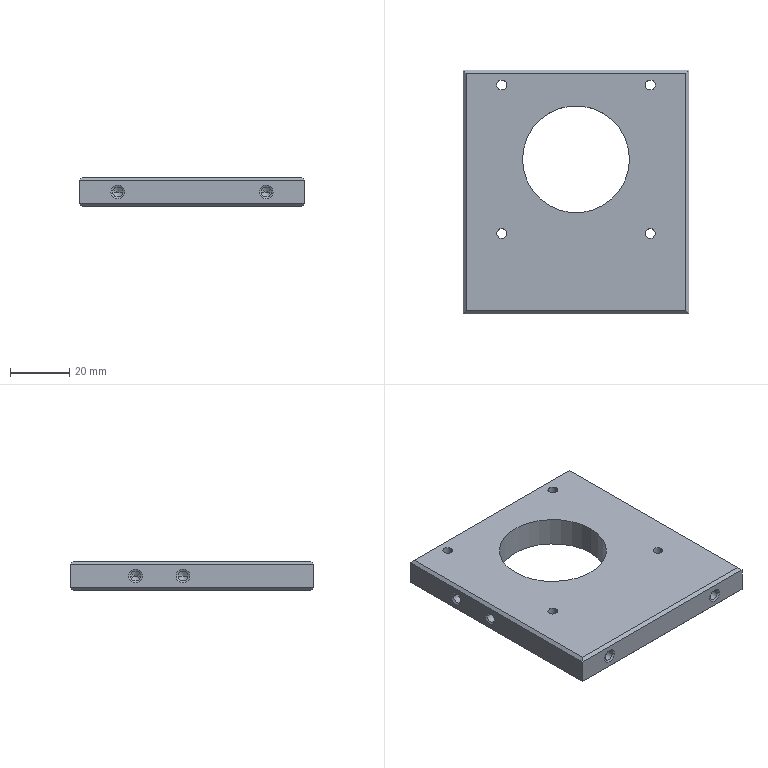Part | NX | 1 solid | 68 faces | box 76 x 82 x 10 mm | volume 50828 mm3 | cone 32 | cylinder 22 | plane 14 | commonest cylinder face diameters 3.3 x20 36 x2